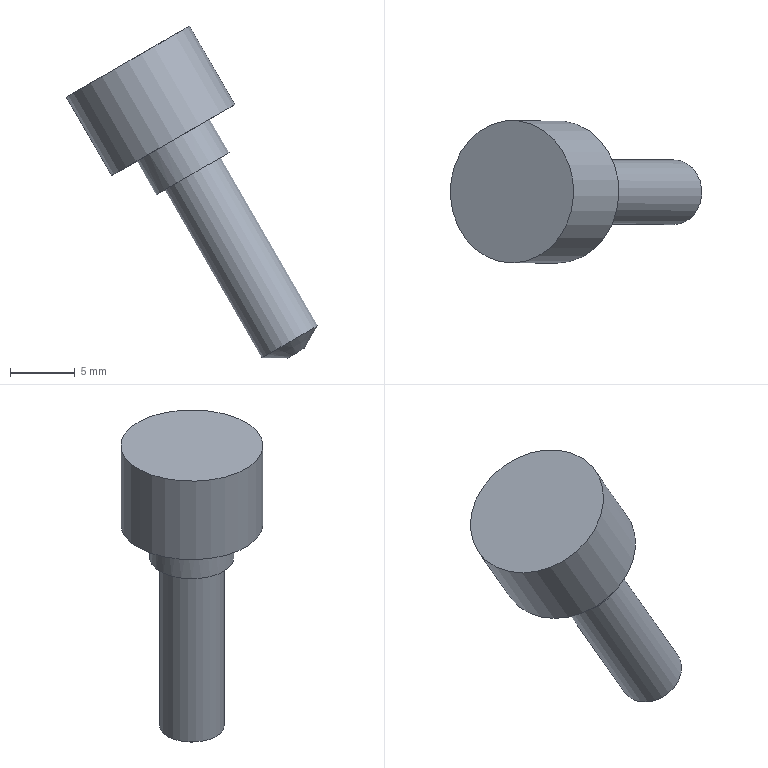Part | STEP file | solid 4 | 1 solid | 8 faces | box 19.428 x 11 x 25.651 mm | volume 1068 mm3 | plane 4 | cylinder 3 | cone 1 | commonest cylinder face diameters 5 x1 6.5 x1 11 x1